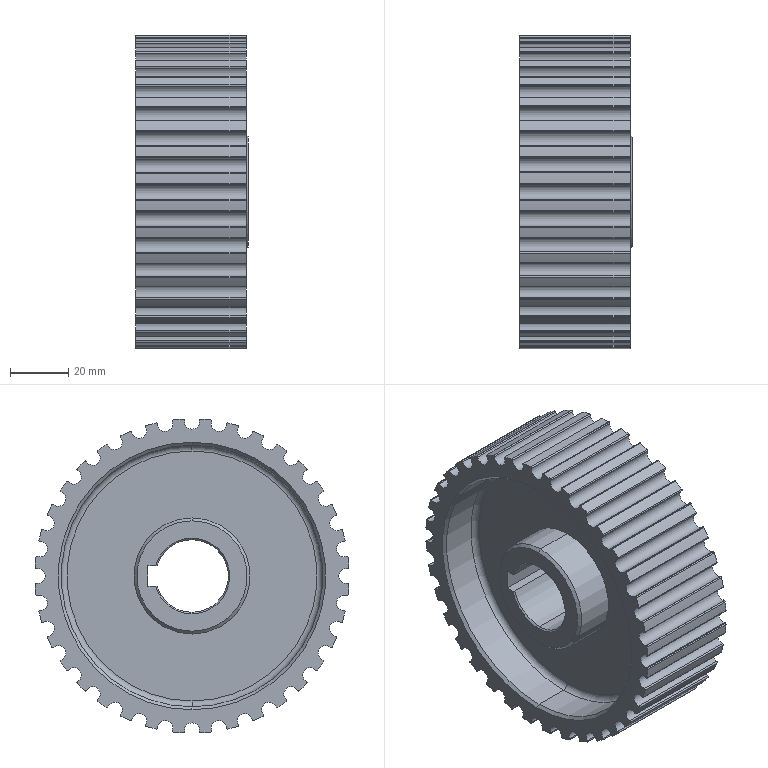Part | SolidWorks | features Chamfer 3, ICE 2, CirPattern 1, Fillet 1, Revolution 1 | 1 solid | 223 faces | box 38.794 x 107.98 x 107.98 mm | volume 165804 mm3 | cylinder 196 | cone 14 | plane 9 | torus 4 | commonest cylinder face diameters 0.8 x92 5.14 x57 108.14 x36 40 x4 90 x4 25 x3